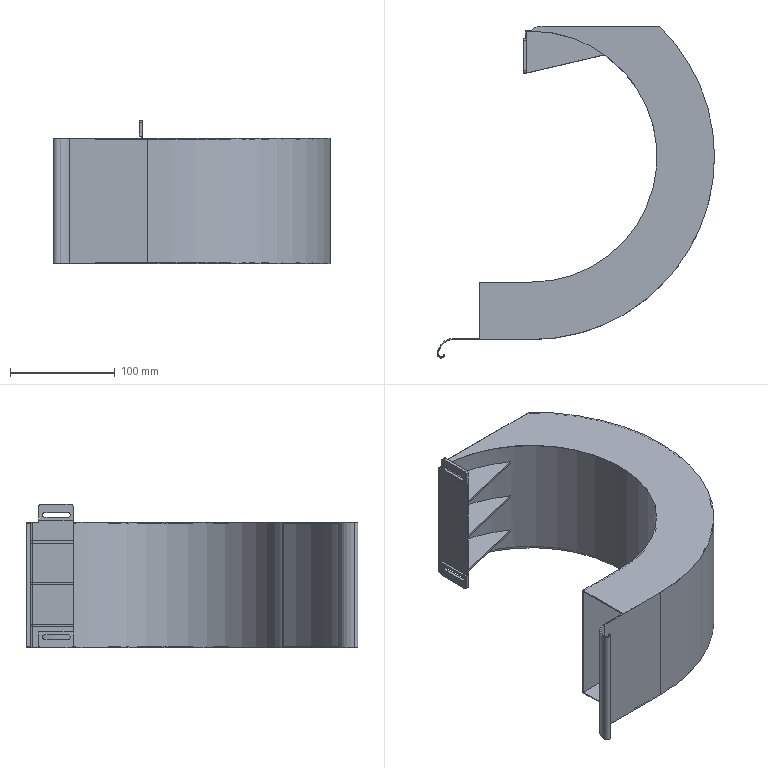Part | STEP file | 11-FG-B07411 | 1 solid | 70 faces | box 265 x 317.5 x 137 mm | volume 178477 mm3 | plane 46 | cylinder 24 | commonest cylinder face diameters 1.473 x4 4 x4 4.5 x4 30 x3 350 x2 3.473 x1